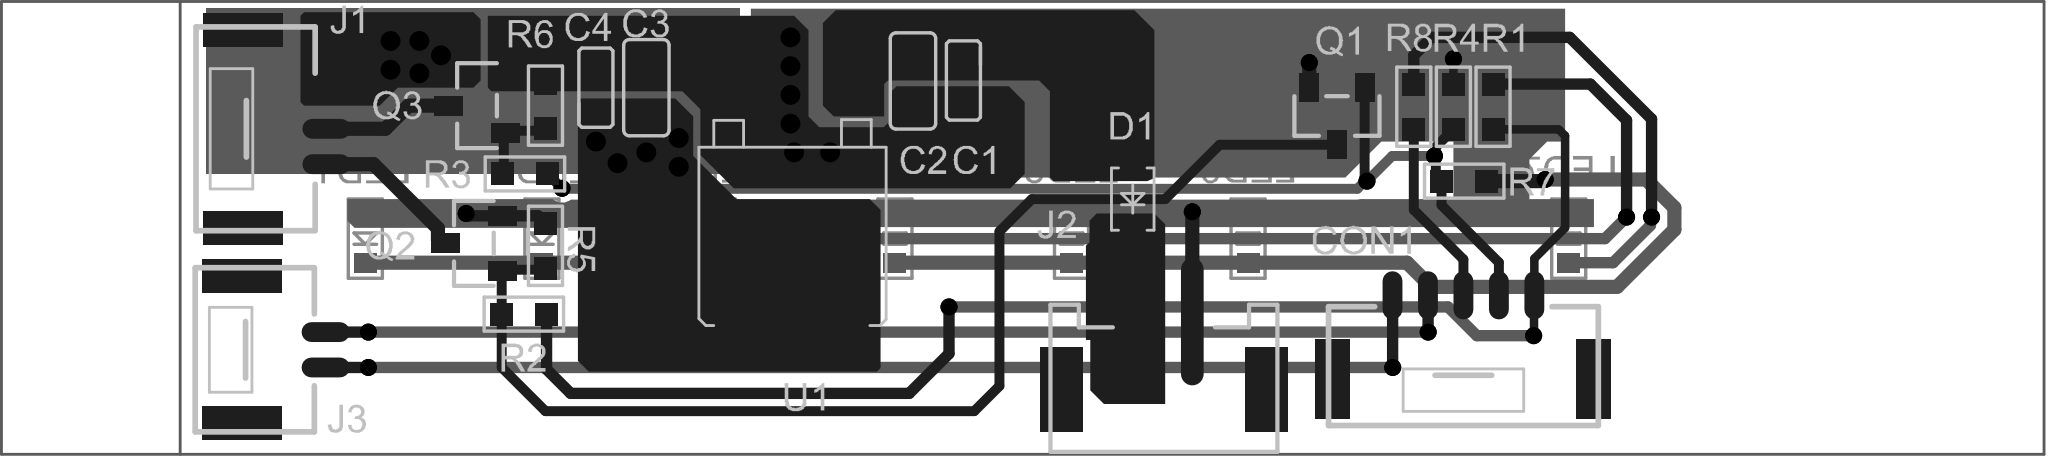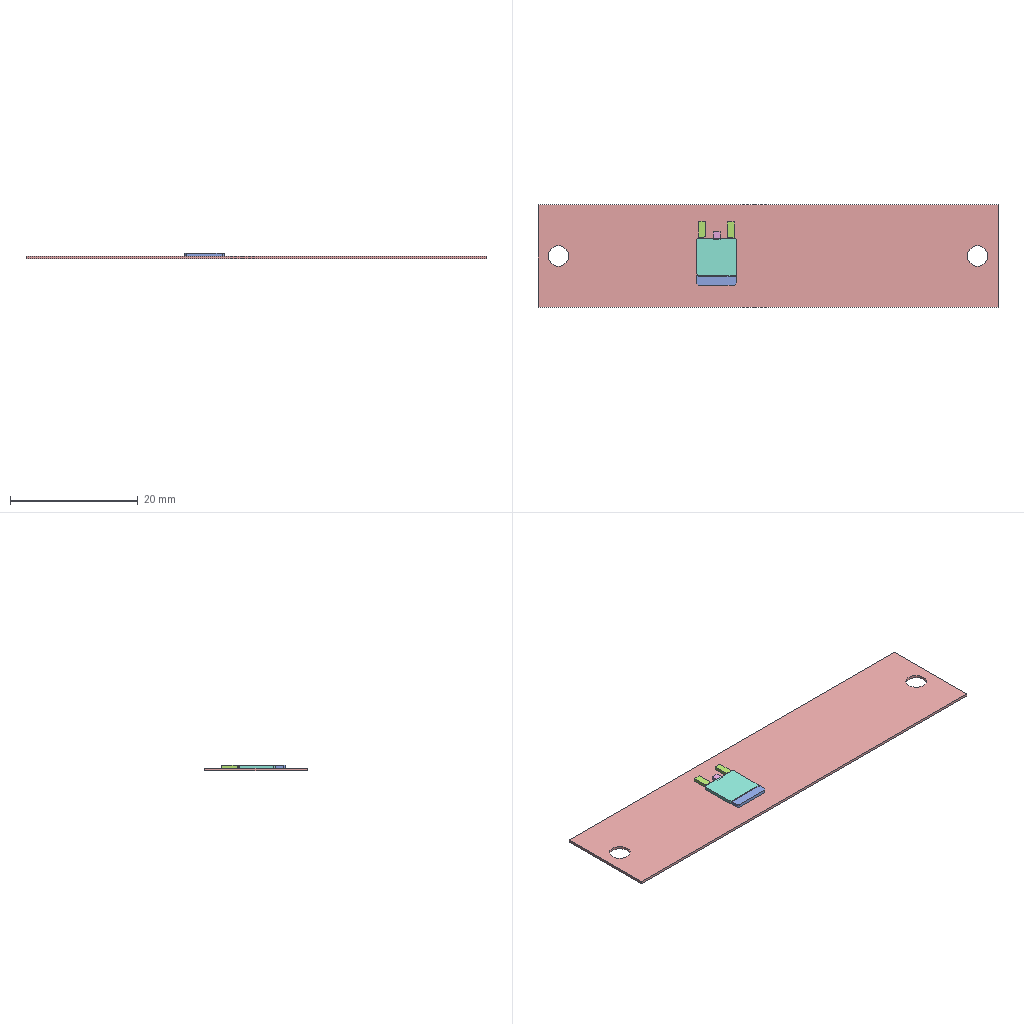Circuit board layout | Altium Designer | box 72 x 16 x 0.9 mm
Layer stack:
# Altium Designer layer stack of  (unit mm; dielectric type: 0 none, 1 core, 2 prepreg, 3 surface material)
index,name,kind,layer,copper_thickness_mm,dielectric_type,dielectric_thickness_mm,dielectric_material,dielectric_constant
0,Top Paste,other,,,,,,
1,Top Overlay,other,,,,,,
2,Top Solder,dielectric,,,3,0.0102,Solder Resist,3.5
3,Top Layer,copper,Top Layer,0.0356,,,,
4,Dielectric 1,dielectric,,,0,0.32,FR-4,4.8
5,Bottom Layer,copper,Bottom Layer,0.0356,,,,
6,Bottom Solder,dielectric,,,3,0.0102,Solder Resist,3.5
7,Bottom Overlay,other,,,,,,
8,Bottom Paste,other,,,,,,
# drill layer pairs: low layer,high layer
drill_pair,Top Layer,Bottom Layer
Part placement:
Designator,Comment,Layer,Footprint,Center-X(mm),Center-Y(mm),Rotation
R8,1K/5%,TopLayer,R0603A,49.784,12.281,270
R7,1K/5%,TopLayer,R0603A,51.562,9.652,0
R6,100K/5%,TopLayer,R0603A,19.177,12.319,270
R5,100K/5%,TopLayer,R0603A,19.177,7.366,270
R4,100K/5%,TopLayer,R0603A,51.181,12.281,90
R3,100K/5%,TopLayer,R0603A,18.453,9.906,180
R2,100K/5%,TopLayer,R0603A,18.415,4.953,180
R1,1K/5%,TopLayer,R0603A,52.578,12.281,90
Q3,CJ2300/SOT23,TopLayer,SOT23-3,16.756,12.319,90
Q2,CJ2300/SOT23,TopLayer,SOT23-3,16.645,7.452,90
Q1,CJ2300/SOT23,TopLayer,SOT23-3,47.076,11.946,180
C4,100nF/50V,TopLayer,C0603A,20.955,12.954,270
C3,10uF/25V,TopLayer,C0805A,22.733,12.954,270
C2,10uF/25V,TopLayer,C0805A,32.131,13.192,90
C1,100nF/50V,TopLayer,C0603A,33.909,13.208,90
U1,78M05/TO252,TopLayer,TO-252-A,27.87,9.585,180
LED6,,BottomLayer,LED0603A,43.942,7.62,90
LED7,,BottomLayer,LED0603A,55.245,7.62,90
LED5,,BottomLayer,LED0603A,37.719,7.62,90
LED4,,BottomLayer,LED0603A,31.496,7.62,90
LED3,,BottomLayer,LED0603A,25.273,7.62,90
LED2,,BottomLayer,LED0603A,19.05,7.62,90
LED1,,BottomLayer,LED0603A,12.827,7.62,90
J3,2PIN,TopLayer,GH1.25-2PIN立贴带扣耐温260℃,9.955,3.693,270
J2,2PIN,TopLayer,HY2.0WT-2A/P_Á¢Ìù´ø¿ÛÄÍÎÂ260¡æ,40.977,3.486,0
J1,3PIN 1.25,TopLayer,GH1.25-3PIN立贴带扣耐温260℃,9.984,11.501,270
CON1,5PIN ribbon cable,TopLayer,GH1.25-5PIN立贴带扣耐温260℃,51.534,4.142,0
D1,SS34/SMA,TopLayer,SOD323,39.878,9.017,90
Pad and via stacks:
# Altium Designer via and pad stacks of  (unit mm). Each distinct definition once, with the count of objects using it.
# via: kind,start_layer,end_layer,hole_mm,diameter_mm,mode(0 simple;1 top-mid-bottom;2 full stack),diameter_per_layer,count,example_net
# pad: kind,layer,hole_mm,hole_type(0 round;1 square;2 slot),plating,top_size,top_shape(1 round;2 rect;3 octagon;9 rounded rect),mid_size,bottom_size,mode,footprint,size_per_layer,count,example
pad,Top Layer,0,0,plated,1.7x0.7,1,1.7x0.7,1.7x0.7,0,GH1.25-3PIN\u00C1\u00A2\u00CC\u00F9\u00B4\u00F8\u00BF\u00DB\u00C4\u00CD\u00CE\u00C2260\u00A1\u00E6,,3,J1.2
pad,Top Layer,0,0,plated,2.8x1.2,2,2.8x1.2,2.8x1.2,0,GH1.25-3PIN\u00C1\u00A2\u00CC\u00F9\u00B4\u00F8\u00BF\u00DB\u00C4\u00CD\u00CE\u00C2260\u00A1\u00E6,,2,J1.0
pad,Top Layer,0,0,plated,1.7x0.7,1,1.7x0.7,1.7x0.7,0,GH1.25-2PIN\u00C1\u00A2\u00CC\u00F9\u00B4\u00F8\u00BF\u00DB\u00C4\u00CD\u00CE\u00C2260\u00A1\u00E6,,2,J3.1
pad,Top Layer,0,0,plated,2.8x1.2,2,2.8x1.2,2.8x1.2,0,GH1.25-2PIN\u00C1\u00A2\u00CC\u00F9\u00B4\u00F8\u00BF\u00DB\u00C4\u00CD\u00CE\u00C2260\u00A1\u00E6,,2,J3.0
pad,Top Layer,0,0,plated,0.8x0.8,2,0.8x0.8,0.8x0.8,0,R0603A,,16,R4.2
pad,Top Layer,0,0,plated,0.7x1,2,0.7x1,0.7x1,0,SOT23-3,,9,Q1.1
pad,Top Layer,0,0,plated,3x1.5,2,3x1.5,3x1.5,0,HY2.0WT-2A/P \u00C1\u00A2\u00CC\u00F9\u00B4\u00F8\u00BF\u00DB\u00C4\u00CD\u00CE\u00C2260\u00A1\u00E6,,2,J2.0
pad,Top Layer,0,0,plated,4.5x0.8,1,4.5x0.8,4.5x0.8,0,HY2.0WT-2A/P \u00C1\u00A2\u00CC\u00F9\u00B4\u00F8\u00BF\u00DB\u00C4\u00CD\u00CE\u00C2260\u00A1\u00E6,,2,J2.1
pad,Top Layer,0,0,plated,0.8x0.8,2,0.8x0.8,0.8x0.8,0,C0603A,,4,C1.1
pad,Top Layer,0,0,plated,1x1.25,2,1x1.25,1x1.25,0,C0805A,,4,C2.1
pad,Top Layer,0,0,plated,1.5x2.5,2,1.5x2.5,1.5x2.5,0,TO-252-A,,1,U1.1
pad,Top Layer,0,0,plated,4.8x5.5,2,4.8x5.5,4.8x5.5,0,TO-252-A,,1,U1.3
pad,Top Layer,0,0,plated,1.8x2.5,2,1.8x2.5,1.8x2.5,0,TO-252-A,,1,U1.2
pad,Top Layer,0,0,plated,2.8x1.2,2,2.8x1.2,2.8x1.2,0,GH1.25-5PIN\u00C1\u00A2\u00CC\u00F9\u00B4\u00F8\u00BF\u00DB\u00C4\u00CD\u00CE\u00C2260\u00A1\u00E6,,2,CON1.0
pad,Top Layer,0,0,plated,1.7x0.7,1,1.7x0.7,1.7x0.7,0,GH1.25-5PIN\u00C1\u00A2\u00CC\u00F9\u00B4\u00F8\u00BF\u00DB\u00C4\u00CD\u00CE\u00C2260\u00A1\u00E6,,5,CON1.5
pad,Top Layer,0,0,plated,0.8x0.7,2,0.8x0.7,0.8x0.7,0,SOD323,,2,D1.1
pad,Bottom Layer,0,0,plated,0.7x0.8,2,0.7x0.8,0.7x0.8,0,LED0603A,,14,LED1.1
via,Top Layer,Bottom Layer,0.4,0.6,0,,16,NetLED4_1
via,Top Layer,Bottom Layer,0.5,0.7,0,,16,DS-
Copper pours:
name,layer,net,type(0 solid;1 hatched;2 none)
DS-_L01_P006,Top Layer,DS-,0
VCC5V_L01_P003,Top Layer,VCC5V,0
VCC5V_L01_P002,Top Layer,VCC5V,0
NETC1_2_L01_P001,Top Layer,NetC1_2,0
P+_L01_P000,Top Layer,P+,0
DS-_L02_P007,Bottom Layer,DS-,0
VCC5V_L02_P005,Bottom Layer,VCC5V,0
DS-_L02_P004,Bottom Layer,DS-,0
Design rules, without the lines most boards share:
# Altium Designer design rules of  (exported by Altium Designer, unit mm)
# columns: name | kind | enabled | priority | scope1 | scope2 | descriptor | typed fields (field=value)
Schematic Supply Nets_1 | 41 | enabled | 1 | InNet('VCC5V') | All | Supply Net(s)(InNet('VCC5V')) |
Schematic Supply Nets | 41 | enabled | 2 | InNet('B-') | All | Supply Net(s)(InNet('B-')) |
NetAntennae | 56 | enabled | 1 | All | All | Net Antennae (Tolerance=0mm) (All) |
SilkToSilkClearance | 55 | enabled | 1 | All | All | Silk to Silk (Clearance=0.01mm) (All),(All) |
SilkToSolderMaskClearance | 54 | enabled | 1 | IsPad | All | Silk To Solder Mask (Clearance=0mm) (IsPad),(All) |
MinimumSolderMaskSliver | 53 | enabled | 1 | All | All | Minimum Solder Mask Sliver (Gap=0.254mm) (All),(All) |
HoleToHoleClearance | 52 | enabled | 1 | All | All | Hole To Hole Clearance (Gap=0.254mm) (All),(All) | gap=0.254
DiffPairsRouting | 51 | enabled | 1 | All | All | Differential Pairs Uncoupled Length using the Gap Constraints (Min=0.254mm) (Max=0.254mm) (Prefered=0.254mm)  and Width Constraints (Min=0.381mm) (Max=0.381mm) (Prefered=0.381mm) (All) |
HoleSize | 42 | enabled | 1 | All | All | Hole Size Constraint (Min=0.025mm) (Max=2.54mm) (All) |
Height | 50 | enabled | 1 | All | All | Height Constraint (Min=0mm) (Max=25.4mm) (Prefered=12.7mm) (All) | min_height=0 max_height=25.4
ComponentClearance | 24 | enabled | 1 | All | All | Component Clearance Constraint ( Horizontal Gap = 0.254mm, Vertical Gap = 0.254mm ) (All),(All)  | gap=0.254
SolderMaskExpansion | 13 | enabled | 1 | All | All | Solder Mask Expansion (Expansion =0.102mm) (All) | expansion=0.1016
PasteMaskExpansion | 14 | enabled | 1 | All | All | Paste Mask Expansion (Expansion =0mm) (All) | expansion=0
RoutingVias | 11 | enabled | 1 | All | All | Routing Via (MinHoleWidth=0.711mm) (MaxHoleWidth=0.711mm) (PreferredHoleWidth=0.711mm) (MinWidth=1.27mm) (MaxWidth=1.27mm) (PreferedWidth=1.27mm) (All) | via_min_hole=0.7112 via_max_hole=0.7112 via_preferred_diameter=1.27 via_preferred_hole=0.7112
RoutingCorners | 10 | enabled | 1 | All | All | Routing Corners (Style=45-Degree) (Min Setback=2.54mm) (Max Setback=2.54mm) (All) |
Width | 2 | enabled | 1 | All | All | Width Constraint (Min=0.254mm) (Max=100mm) (Preferred=0.254mm) (All) |
PolygonConnect | 20 | enabled | 1 | All | All | Polygon Connect Rule(Direct Connect )(Conductor Width=0.254mm) (Relief Angle=90 Angle) (Entries=4) (Air Gap Width=0.254mm) (All),(All) | connect_style(0=relief,1=direct,2=none)=1 relief_conductor_width=0.254 relief_entries=4
PlaneClearance | 12 | enabled | 1 | All | All | Power Plane Clearance (Clearance =0.508mm) (All) | clearance=0.508
PlaneConnect | 6 | enabled | 1 | All | All | Power Plane Connect Rule(Relief Connect )(Expansion=0.508mm) (Conductor Width=0.254mm) (Air Gap=0.254mm) (Entries=4) (All) | relief_conductor_width=0.254 relief_entries=4 relief_expansion=0.508
Clearance | 0 | enabled | 1 | All | All | Clearance Constraint (Gap=0.2mm) (All),(All) | gap=0.2